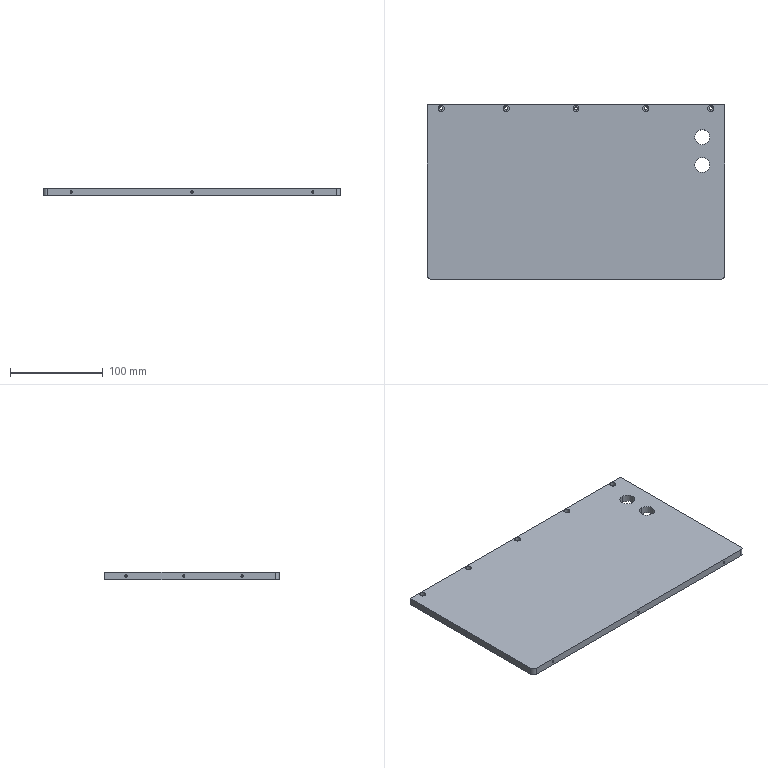CAM job | Mastercam | 3-axis milling, drilling | part box 320 x 188 x 8 mm | stock box 325 x 193 x 8 mm
Tools:
tool_number,name,type,diameter_mm,corner_radius_mm,flutes,flute_length_mm,overall_length_mm,shoulder_length_mm,holder_diameter_mm,length_offset,diameter_offset,default_rpm,default_feed_mm_min,default_plunge_mm_min,coolant
1,10 Flat End Mill,end mill,10,0,4,25,75,25,50,1,1,8000,2000,600,COOL_OFF
2,10 Flat End Mill,end mill,10,0,4,25,75,25,50,2,2,8000,1000,600,COOL_OFF
3,6 Chamfer Mill,chamfer mill,6,0,4,25,75,30,50,3,3,5000,1000,600,COOL_OFF
4,7.94 Center Drill,drill,7.94,0,2,7.302,54,7.302,50,4,4,2000,200,600,COOL_OFF
5,3.4 Drill,drill,3.4,0,2,25,50,40,50,5,5,1765,200,600,COOL_OFF
6,4 Flat End Mill,end mill,4,0,4,25,75,25,50,6,6,8000,1000,600,COOL_OFF
Operations:
seq,operation,operation_type,tool_number,tool_name,tool_diameter_mm,spindle_rpm,feed_mm_min,plunge_mm_min,retract_mm_min,cycle_time_s,wcs,posted,nc_file
1,Contour (2D) - [WCS: Top] - [Tplane: Top],Contour,1,10 Flat End Mill,10,8000,2000,600,1200,9.837,Top,yes,1.nc
2,Contour (2D) - [WCS: Top] - [Tplane: Top],Contour,1,10 Flat End Mill,10,8000,2000,600,1200,33.879,Top,yes,1.nc
3,Contour (Ramp) - [WCS: Top] - [Tplane: Top],Contour,1,10 Flat End Mill,10,8000,3000,600,1200,7.136,Top,yes,1.nc
4,Contour (2D) - [WCS: Top] - [Tplane: Top],Contour,2,10 Flat End Mill,10,8000,1000,600,1200,28.181,Top,yes,1.nc
5,Contour (2D) - [WCS: Top] - [Tplane: Top],Contour,2,10 Flat End Mill,10,8000,1000,600,1200,4.698,Top,yes,1.nc
6,Model Chamfer - [WCS: Top] - [Tplane: Top],ModelChamfer,3,6 Chamfer Mill,6,5000,1000,600,1200,33.243,Top,yes,1.nc
7,Contour (2D) - [WCS: Top] - [Tplane: Top],Contour,1,10 Flat End Mill,10,8000,2000,600,1200,48.994,Top,yes,2.nc
8,Drill/Counterbore - [WCS: Top] - [Tplane: Top],Drill,4,7.94 Center Drill,7.94,2000,200,600,1200,3.48,Top,yes,2.nc
9,Peck Drill - [WCS: Top] - [Tplane: Top],Drill,5,3.4 Drill,3.4,1765,200,600,1200,18.636,Top,yes,2.nc
10,Contour (Ramp) - [WCS: Top] - [Tplane: Top],Contour,6,4 Flat End Mill,4,8000,1000,600,1200,24.001,Top,yes,2.nc
11,Contour (2D) - [WCS: Top] - [Tplane: Top],Contour,2,10 Flat End Mill,10,8000,1000,600,1200,42.324,Top,yes,2.nc
12,Model Chamfer - [WCS: Top] - [Tplane: Top],ModelChamfer,3,6 Chamfer Mill,6,5000,1000,600,1200,49.416,Top,yes,2.nc